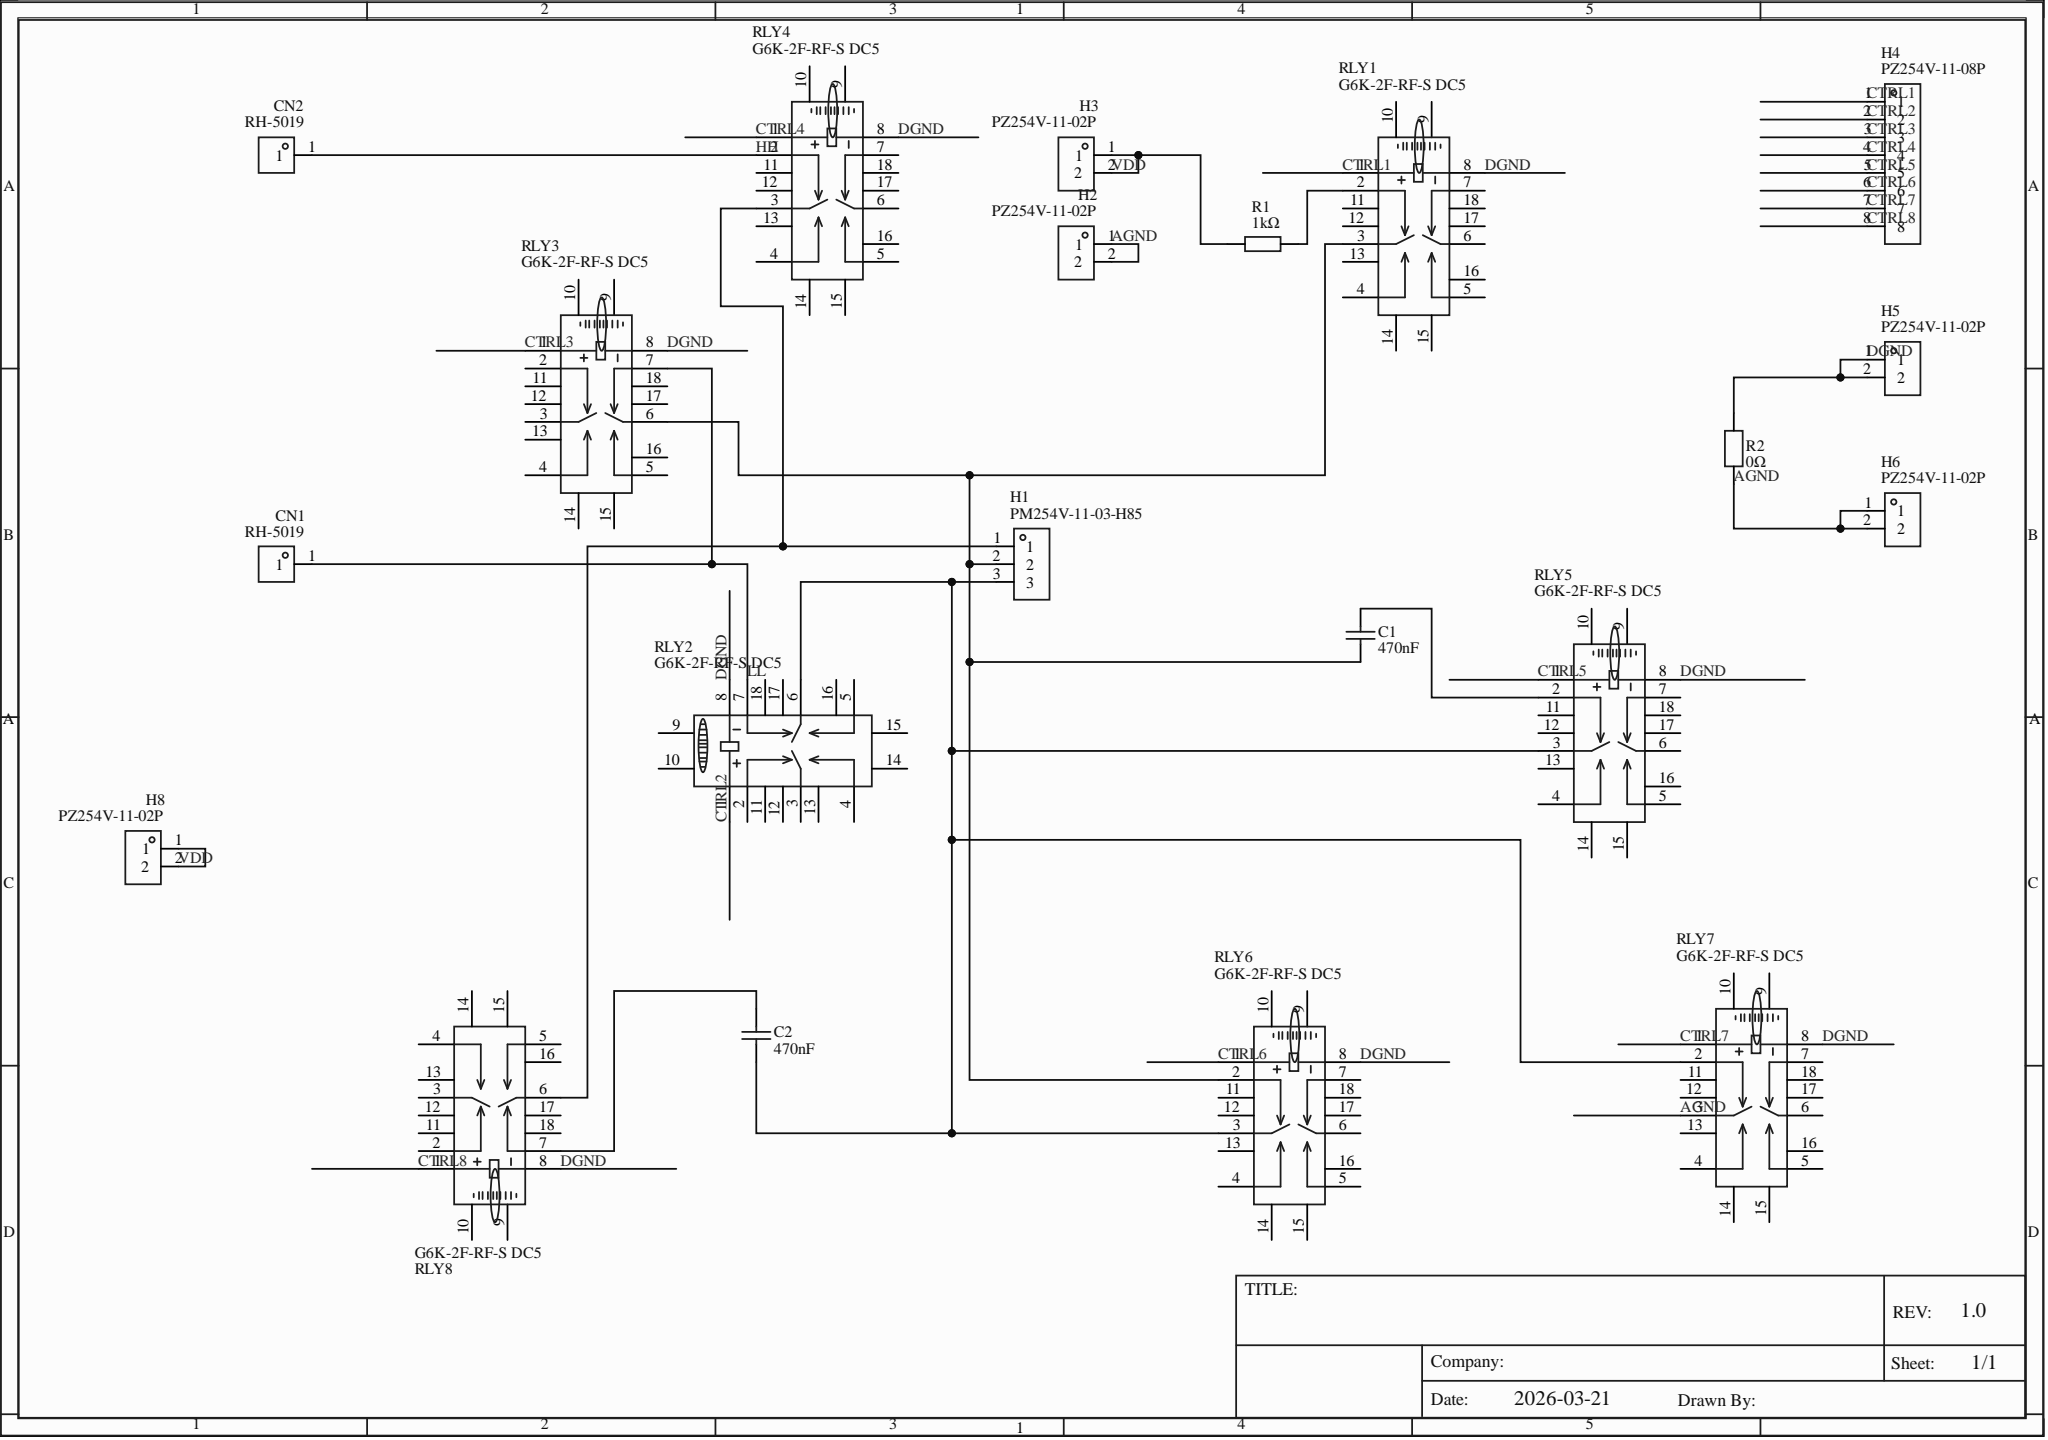Circuit board | Altium Designer | 21 parts | 19 nets
Bill of materials:
Comment,Description,Designator,Footprint,LibRef,Quantity
"470nF","","C1, C2","C0805","CL21B474KBFNNNE","2"
"RH-5019","","CN1, CN2","TESTPOINT-SMD_L3.8-W2.0_RH-5019","RH-5019","2"
"PM254V-11-03-H85","","H1","HDR-TH_3P-P2.54-V-F","PM254V-11-03-H85","1"
"PZ254V-11-02P","","H2, H3, H5, H6, H8","HDR-TH_2P-P2.54-V-M","PZ254V-11-02P","5"
"PZ254V-11-08P","","H4","HDR-TH_8P-P2.54-V-M","PZ254V-11-08P","1"
"1kΩ","","R1","R1210","1210W2J0102T5E","1"
"0Ω","","R2","R1206","RE1206F1R000","1"
"G6K-2F-RF-S DC5","","RLY1, RLY2, RLY3, RLY4, RLY5, RLY6, RLY7, RLY8","RELAY-SMD_G6K-2F-RF-S-DC12","G6K-2F-RF-S DC5","8"
Netlist (Protel format):
[
C1
C0805
470nF



]
[
C2
C0805
470nF



]
[
CN1
TESTPOINT-SMD_L3.8-W2.0_RH-5019
RH-5019



]
[
CN2
TESTPOINT-SMD_L3.8-W2.0_RH-5019
RH-5019



]
[
H1
HDR-TH_3P-P2.54-V-F
PM254V-11-03-H85



]
[
H2
HDR-TH_2P-P2.54-V-M
PZ254V-11-02P



]
[
H3
HDR-TH_2P-P2.54-V-M
PZ254V-11-02P



]
[
H4
HDR-TH_8P-P2.54-V-M
PZ254V-11-08P



]
[
H5
HDR-TH_2P-P2.54-V-M
PZ254V-11-02P



]
[
H6
HDR-TH_2P-P2.54-V-M
PZ254V-11-02P



]
[
H8
HDR-TH_2P-P2.54-V-M
PZ254V-11-02P



]
[
R1
R1210
1kΩ



]
[
R2
R1206
0Ω



]
[
RLY1
RELAY-SMD_G6K-2F-RF-S-DC12
G6K-2F-RF-S DC5



]
[
RLY2
RELAY-SMD_G6K-2F-RF-S-DC12
G6K-2F-RF-S DC5



]
[
RLY3
RELAY-SMD_G6K-2F-RF-S-DC12
G6K-2F-RF-S DC5



]
[
RLY4
RELAY-SMD_G6K-2F-RF-S-DC12
G6K-2F-RF-S DC5



]
[
RLY5
RELAY-SMD_G6K-2F-RF-S-DC12
G6K-2F-RF-S DC5



]
[
RLY6
RELAY-SMD_G6K-2F-RF-S-DC12
G6K-2F-RF-S DC5



]
[
RLY7
RELAY-SMD_G6K-2F-RF-S-DC12
G6K-2F-RF-S DC5



]
[
RLY8
RELAY-SMD_G6K-2F-RF-S-DC12
G6K-2F-RF-S DC5



]
(
VDD
H3-1
H3-2
H8-1
H8-2
R1-1
)
(
NetR1_2
R1-2
RLY1-2
)
(
NetH1_1
H1-1
RLY4-3
RLY8-6
)
(
NetC2_2
C2-2
RLY8-7
)
(
NetC2_1
C2-1
H1-3
RLY2-6
RLY5-3
RLY6-3
RLY7-2
)
(
NetC1_2
C1-2
RLY5-2
)
(
NetC1_1
C1-1
H1-2
RLY1-3
RLY3-6
RLY6-2
)
(
LL
CN1-1
RLY2-7
RLY3-7
)
(
HH
CN2-1
RLY4-2
)
(
DGND
H5-1
H5-2
R2-2
RLY1-8
RLY2-8
RLY3-8
RLY4-8
RLY5-8
RLY6-8
RLY7-8
RLY8-8
)
(
CTRL8
H4-8
RLY8-1
)
(
CTRL7
H4-7
RLY7-1
)
(
CTRL6
H4-6
RLY6-1
)
(
CTRL5
H4-5
RLY5-1
)
(
CTRL4
H4-4
RLY4-1
)
(
CTRL3
H4-3
RLY3-1
)
(
CTRL2
H4-2
RLY2-1
)
(
CTRL1
H4-1
RLY1-1
)
(
AGND
H2-1
H2-2
H6-1
H6-2
R2-1
RLY7-3
)